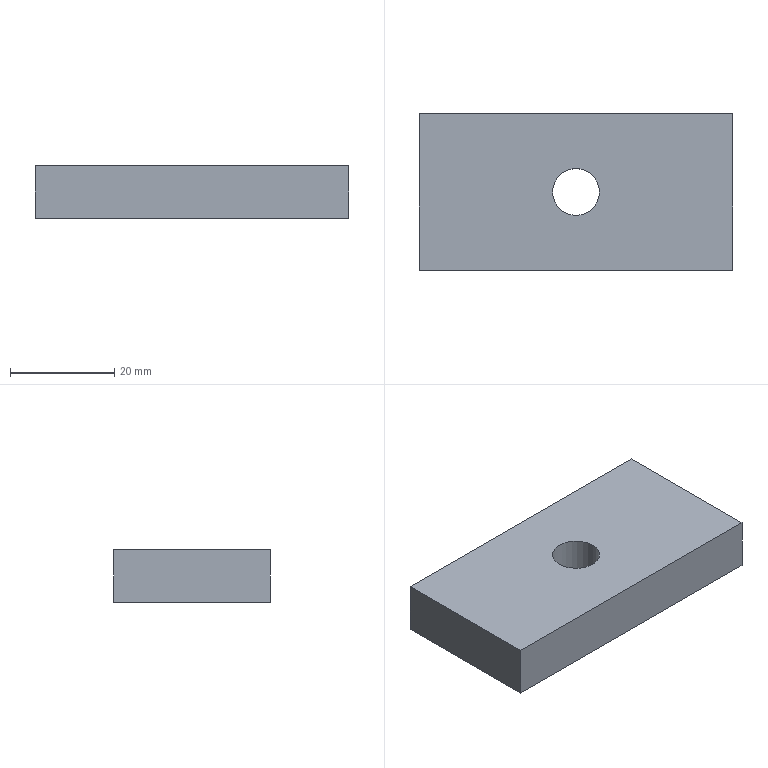Part | NX | features solid 2 | 1 solid | 7 faces | box 60 x 30 x 10 mm | volume 17364 mm3 | plane 6 | cylinder 1 | commonest cylinder face diameters 9 x1
STEP:
#1=CARTESIAN_POINT('',(630.5,-240.,10.));
#2=VERTEX_POINT('',#1);
#3=CARTESIAN_POINT('',(635.,-240.,10.));
#4=DIRECTION('',(0.,0.,-1.));
#5=DIRECTION('',(-1.,0.,0.));
#6=AXIS2_PLACEMENT_3D('',#3,#4,#5);
#7=CIRCLE('',#6,4.5);
#8=EDGE_CURVE('',#2,#2,#7,.T.);
#9=ORIENTED_EDGE('',*,*,#8,.T.);
#10=EDGE_LOOP('',(#9));
#11=FACE_BOUND('',#10,.T.);
#12=CARTESIAN_POINT('',(630.5,-240.,20.));
#13=VERTEX_POINT('',#12);
#14=CARTESIAN_POINT('',(635.,-240.,20.));
#15=DIRECTION('',(0.,0.,-1.));
#16=DIRECTION('',(-1.,0.,0.));
#17=AXIS2_PLACEMENT_3D('',#14,#15,#16);
#18=CIRCLE('',#17,4.5);
#19=EDGE_CURVE('',#13,#13,#18,.T.);
#20=ORIENTED_EDGE('',*,*,#19,.F.);
#21=EDGE_LOOP('',(#20));
#22=FACE_BOUND('',#21,.T.);
#23=CARTESIAN_POINT('',(635.,-240.,30.));
#24=DIRECTION('',(0.,0.,-1.));
#25=DIRECTION('',(-1.,0.,0.));
#26=AXIS2_PLACEMENT_3D('',#23,#24,#25);
#27=CYLINDRICAL_SURFACE('',#26,4.5);
#28=ADVANCED_FACE('',(#11,#22),#27,.F.);
#29=CARTESIAN_POINT('',(665.,-255.,10.));
#30=VERTEX_POINT('',#29);
#31=CARTESIAN_POINT('',(605.,-255.,10.));
#32=VERTEX_POINT('',#31);
#33=CARTESIAN_POINT('',(675.,-255.,10.));
#34=DIRECTION('',(1.,0.,0.));
#35=VECTOR('',#34,1000.);
#36=LINE('',#33,#35);
#37=EDGE_CURVE('',#30,#32,#36,.F.);
#38=ORIENTED_EDGE('',*,*,#37,.F.);
#39=CARTESIAN_POINT('',(665.,-255.,20.));
#40=VERTEX_POINT('',#39);
#41=CARTESIAN_POINT('',(665.,-255.,-60.));
#42=DIRECTION('',(0.,0.,-1.));
#43=VECTOR('',#42,1000.);
#44=LINE('',#41,#43);
#45=EDGE_CURVE('',#40,#30,#44,.T.);
#46=ORIENTED_EDGE('',*,*,#45,.F.);
#47=CARTESIAN_POINT('',(605.,-255.,20.));
#48=VERTEX_POINT('',#47);
#49=CARTESIAN_POINT('',(675.,-255.,20.));
#50=DIRECTION('',(1.,0.,0.));
#51=VECTOR('',#50,1000.);
#52=LINE('',#49,#51);
#53=EDGE_CURVE('',#40,#48,#52,.F.);
#54=ORIENTED_EDGE('',*,*,#53,.T.);
#55=CARTESIAN_POINT('',(605.,-255.,-60.));
#56=DIRECTION('',(0.,0.,1.));
#57=VECTOR('',#56,1000.);
#58=LINE('',#55,#57);
#59=EDGE_CURVE('',#48,#32,#58,.F.);
#60=ORIENTED_EDGE('',*,*,#59,.T.);
#61=EDGE_LOOP('',(#38,#46,#54,#60));
#62=FACE_BOUND('',#61,.T.);
#63=CARTESIAN_POINT('',(690.,-255.,-60.));
#64=DIRECTION('',(0.,1.,0.));
#65=DIRECTION('',(0.,0.,1.));
#66=AXIS2_PLACEMENT_3D('',#63,#64,#65);
#67=PLANE('',#66);
#68=ADVANCED_FACE('',(#62),#67,.F.);
#69=CARTESIAN_POINT('',(605.,-225.,20.));
#70=VERTEX_POINT('',#69);
#71=CARTESIAN_POINT('',(605.,-225.,10.));
#72=VERTEX_POINT('',#71);
#73=CARTESIAN_POINT('',(605.,-225.,-60.));
#74=DIRECTION('',(0.,0.,1.));
#75=VECTOR('',#74,1000.);
#76=LINE('',#73,#75);
#77=EDGE_CURVE('',#70,#72,#76,.F.);
#78=ORIENTED_EDGE('',*,*,#77,.T.);
#79=CARTESIAN_POINT('',(605.,-255.,10.));
#80=DIRECTION('',(0.,1.,0.));
#81=VECTOR('',#80,1000.);
#82=LINE('',#79,#81);
#83=EDGE_CURVE('',#32,#72,#82,.T.);
#84=ORIENTED_EDGE('',*,*,#83,.F.);
#85=ORIENTED_EDGE('',*,*,#59,.F.);
#86=CARTESIAN_POINT('',(605.,-255.,20.));
#87=DIRECTION('',(0.,1.,0.));
#88=VECTOR('',#87,1000.);
#89=LINE('',#86,#88);
#90=EDGE_CURVE('',#48,#70,#89,.T.);
#91=ORIENTED_EDGE('',*,*,#90,.T.);
#92=EDGE_LOOP('',(#78,#84,#85,#91));
#93=FACE_BOUND('',#92,.T.);
#94=CARTESIAN_POINT('',(605.,-255.,-60.));
#95=DIRECTION('',(1.,0.,0.));
#96=DIRECTION('',(0.,0.,-1.));
#97=AXIS2_PLACEMENT_3D('',#94,#95,#96);
#98=PLANE('',#97);
#99=ADVANCED_FACE('',(#93),#98,.F.);
#100=CARTESIAN_POINT('',(665.,-225.,20.));
#101=VERTEX_POINT('',#100);
#102=CARTESIAN_POINT('',(675.,-225.,20.));
#103=DIRECTION('',(1.,0.,0.));
#104=VECTOR('',#103,1000.);
#105=LINE('',#102,#104);
#106=EDGE_CURVE('',#101,#70,#105,.F.);
#107=ORIENTED_EDGE('',*,*,#106,.F.);
#108=CARTESIAN_POINT('',(665.,-225.,10.));
#109=VERTEX_POINT('',#108);
#110=CARTESIAN_POINT('',(665.,-225.,-10.));
#111=DIRECTION('',(0.,0.,-1.));
#112=VECTOR('',#111,1000.);
#113=LINE('',#110,#112);
#114=EDGE_CURVE('',#109,#101,#113,.F.);
#115=ORIENTED_EDGE('',*,*,#114,.F.);
#116=CARTESIAN_POINT('',(675.,-225.,10.));
#117=DIRECTION('',(1.,0.,0.));
#118=VECTOR('',#117,1000.);
#119=LINE('',#116,#118);
#120=EDGE_CURVE('',#109,#72,#119,.F.);
#121=ORIENTED_EDGE('',*,*,#120,.T.);
#122=ORIENTED_EDGE('',*,*,#77,.F.);
#123=EDGE_LOOP('',(#107,#115,#121,#122));
#124=FACE_BOUND('',#123,.T.);
#125=CARTESIAN_POINT('',(690.,-225.,-60.));
#126=DIRECTION('',(0.,1.,0.));
#127=DIRECTION('',(0.,0.,1.));
#128=AXIS2_PLACEMENT_3D('',#125,#126,#127);
#129=PLANE('',#128);
#130=ADVANCED_FACE('',(#124),#129,.T.);
#131=ORIENTED_EDGE('',*,*,#120,.F.);
#132=CARTESIAN_POINT('',(665.,205.,10.));
#133=DIRECTION('',(0.,1.,0.));
#134=VECTOR('',#133,1000.);
#135=LINE('',#132,#134);
#136=EDGE_CURVE('',#109,#30,#135,.F.);
#137=ORIENTED_EDGE('',*,*,#136,.T.);
#138=ORIENTED_EDGE('',*,*,#37,.T.);
#139=ORIENTED_EDGE('',*,*,#83,.T.);
#140=EDGE_LOOP('',(#131,#137,#138,#139));
#141=FACE_BOUND('',#140,.T.);
#142=ORIENTED_EDGE('',*,*,#8,.F.);
#143=EDGE_LOOP('',(#142));
#144=FACE_BOUND('',#143,.T.);
#145=CARTESIAN_POINT('',(675.,205.,10.));
#146=DIRECTION('',(0.,0.,-1.));
#147=DIRECTION('',(-1.,0.,0.));
#148=AXIS2_PLACEMENT_3D('',#145,#146,#147);
#149=PLANE('',#148);
#150=ADVANCED_FACE('',(#141,#144),#149,.T.);
#151=ORIENTED_EDGE('',*,*,#19,.T.);
#152=EDGE_LOOP('',(#151));
#153=FACE_BOUND('',#152,.T.);
#154=CARTESIAN_POINT('',(665.,205.,20.));
#155=DIRECTION('',(0.,-1.,0.));
#156=VECTOR('',#155,1000.);
#157=LINE('',#154,#156);
#158=EDGE_CURVE('',#40,#101,#157,.F.);
#159=ORIENTED_EDGE('',*,*,#158,.T.);
#160=ORIENTED_EDGE('',*,*,#106,.T.);
#161=ORIENTED_EDGE('',*,*,#90,.F.);
#162=ORIENTED_EDGE('',*,*,#53,.F.);
#163=EDGE_LOOP('',(#159,#160,#161,#162));
#164=FACE_BOUND('',#163,.T.);
#165=CARTESIAN_POINT('',(675.,205.,20.));
#166=DIRECTION('',(0.,0.,-1.));
#167=DIRECTION('',(-1.,0.,0.));
#168=AXIS2_PLACEMENT_3D('',#165,#166,#167);
#169=PLANE('',#168);
#170=ADVANCED_FACE('',(#153,#164),#169,.F.);
#171=ORIENTED_EDGE('',*,*,#136,.F.);
#172=ORIENTED_EDGE('',*,*,#114,.T.);
#173=ORIENTED_EDGE('',*,*,#158,.F.);
#174=ORIENTED_EDGE('',*,*,#45,.T.);
#175=EDGE_LOOP('',(#171,#172,#173,#174));
#176=FACE_BOUND('',#175,.T.);
#177=CARTESIAN_POINT('',(665.,205.,-10.));
#178=DIRECTION('',(1.,0.,0.));
#179=DIRECTION('',(0.,0.,-1.));
#180=AXIS2_PLACEMENT_3D('',#177,#178,#179);
#181=PLANE('',#180);
#182=ADVANCED_FACE('',(#176),#181,.T.);
#183=CLOSED_SHELL('',(#28,#68,#99,#130,#150,#170,#182));
#184=MANIFOLD_SOLID_BREP('',#183);
#185=(LENGTH_UNIT()NAMED_UNIT(*)SI_UNIT(.MILLI.,.METRE.));
#186=UNCERTAINTY_MEASURE_WITH_UNIT(LENGTH_MEASURE(0.00001),#185,'','');
#187=(NAMED_UNIT(*)PLANE_ANGLE_UNIT()SI_UNIT($,.RADIAN.));
#188=(NAMED_UNIT(*)SI_UNIT($,.STERADIAN.)SOLID_ANGLE_UNIT());
#189=(GEOMETRIC_REPRESENTATION_CONTEXT(3)GLOBAL_UNCERTAINTY_ASSIGNED_CONTEXT((#186))GLOBAL_UNIT_ASSIGNED_CONTEXT((#185,#187,#188))REPRESENTATION_CONTEXT('',''));
#190=ADVANCED_BREP_SHAPE_REPRESENTATION('',(#184),#189);